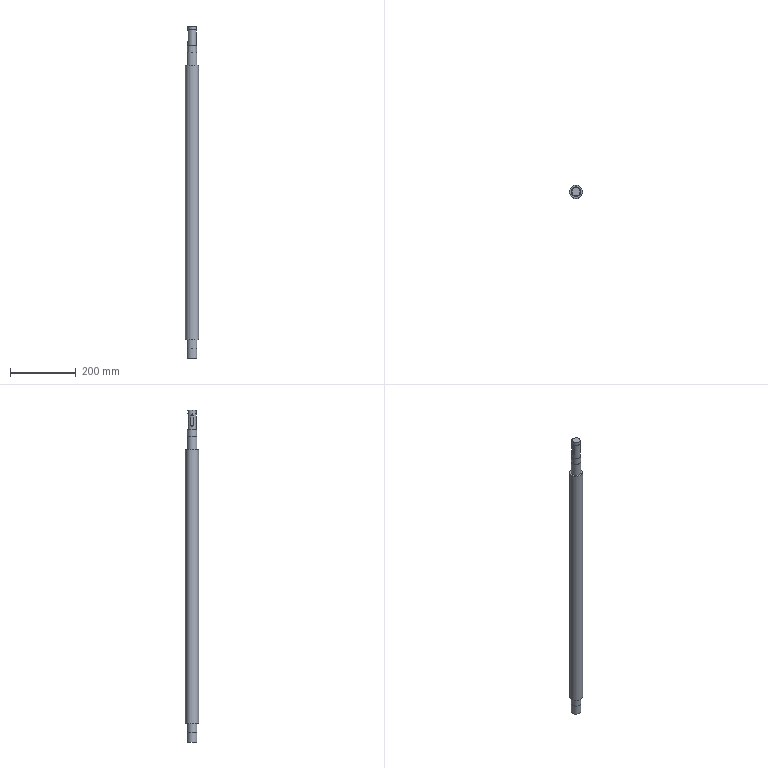Part | NX | features EXTRUDE 8, DATUM_CSYS 5, SKETCH 4, EXTRACT_DATUM_AXIS 2, CPROJ 1, DATUM_PLANE 1, EXTRACT_DATUM_PLANE 1, LINKED_POINT 1 | 3 solids | 24 faces | volume 1157120 mm3 | plane 14 | cylinder 10 | commonest cylinder face diameters 30 x3 8 x2 25 x2 23.2 x1 28 x1 40 x1
STEP:
#1=CARTESIAN_POINT('',(20.,0.,-405.));
#2=VERTEX_POINT('',#1);
#3=CARTESIAN_POINT('',(0.,0.,-405.));
#4=DIRECTION('',(0.,0.,1.));
#5=DIRECTION('',(1.,0.,0.));
#6=AXIS2_PLACEMENT_3D('',#3,#4,#5);
#7=CIRCLE('',#6,20.);
#8=EDGE_CURVE('',#2,#2,#7,.T.);
#9=ORIENTED_EDGE('',*,*,#8,.T.);
#10=EDGE_LOOP('',(#9));
#11=FACE_BOUND('',#10,.T.);
#12=CARTESIAN_POINT('',(20.,0.,430.));
#13=VERTEX_POINT('',#12);
#14=CARTESIAN_POINT('',(0.,0.,430.));
#15=DIRECTION('',(0.,0.,1.));
#16=DIRECTION('',(1.,0.,0.));
#17=AXIS2_PLACEMENT_3D('',#14,#15,#16);
#18=CIRCLE('',#17,20.);
#19=EDGE_CURVE('',#13,#13,#18,.T.);
#20=ORIENTED_EDGE('',*,*,#19,.F.);
#21=EDGE_LOOP('',(#20));
#22=FACE_BOUND('',#21,.T.);
#23=CARTESIAN_POINT('',(0.,0.,430.));
#24=DIRECTION('',(0.,0.,-1.));
#25=DIRECTION('',(-1.,0.,0.));
#26=AXIS2_PLACEMENT_3D('',#23,#24,#25);
#27=CYLINDRICAL_SURFACE('',#26,20.);
#28=ADVANCED_FACE('',(#11,#22),#27,.T.);
#29=ORIENTED_EDGE('',*,*,#19,.T.);
#30=EDGE_LOOP('',(#29));
#31=FACE_BOUND('',#30,.T.);
#32=CARTESIAN_POINT('',(0.,0.,430.));
#33=DIRECTION('',(0.,0.,1.));
#34=DIRECTION('',(1.,0.,0.));
#35=AXIS2_PLACEMENT_3D('',#32,#33,#34);
#36=PLANE('',#35);
#37=ADVANCED_FACE('',(#31),#36,.T.);
#38=CARTESIAN_POINT('',(-15.,0.,-405.));
#39=VERTEX_POINT('',#38);
#40=CARTESIAN_POINT('',(0.,0.,-405.));
#41=DIRECTION('',(0.,0.,-1.));
#42=DIRECTION('',(-1.,0.,0.));
#43=AXIS2_PLACEMENT_3D('',#40,#41,#42);
#44=CIRCLE('',#43,15.);
#45=EDGE_CURVE('',#39,#39,#44,.F.);
#46=ORIENTED_EDGE('',*,*,#45,.F.);
#47=EDGE_LOOP('',(#46));
#48=FACE_BOUND('',#47,.T.);
#49=CARTESIAN_POINT('',(-15.,0.,-430.));
#50=VERTEX_POINT('',#49);
#51=CARTESIAN_POINT('',(0.,0.,-430.));
#52=DIRECTION('',(0.,0.,-1.));
#53=DIRECTION('',(-1.,0.,0.));
#54=AXIS2_PLACEMENT_3D('',#51,#52,#53);
#55=CIRCLE('',#54,15.);
#56=EDGE_CURVE('',#50,#50,#55,.T.);
#57=ORIENTED_EDGE('',*,*,#56,.F.);
#58=EDGE_LOOP('',(#57));
#59=FACE_BOUND('',#58,.T.);
#60=CARTESIAN_POINT('',(0.,0.,-405.));
#61=DIRECTION('',(0.,0.,-1.));
#62=DIRECTION('',(-1.,0.,0.));
#63=AXIS2_PLACEMENT_3D('',#60,#61,#62);
#64=CYLINDRICAL_SURFACE('',#63,15.);
#65=ADVANCED_FACE('',(#48,#59),#64,.T.);
#66=ORIENTED_EDGE('',*,*,#8,.F.);
#67=EDGE_LOOP('',(#66));
#68=FACE_BOUND('',#67,.T.);
#69=ORIENTED_EDGE('',*,*,#45,.T.);
#70=EDGE_LOOP('',(#69));
#71=FACE_BOUND('',#70,.T.);
#72=CARTESIAN_POINT('',(0.,0.,-405.));
#73=DIRECTION('',(0.,0.,1.));
#74=DIRECTION('',(1.,0.,0.));
#75=AXIS2_PLACEMENT_3D('',#72,#73,#74);
#76=PLANE('',#75);
#77=ADVANCED_FACE('',(#68,#71),#76,.F.);
#78=ORIENTED_EDGE('',*,*,#56,.T.);
#79=EDGE_LOOP('',(#78));
#80=FACE_BOUND('',#79,.T.);
#81=CARTESIAN_POINT('',(0.,0.,-430.));
#82=DIRECTION('',(0.,0.,1.));
#83=DIRECTION('',(1.,0.,0.));
#84=AXIS2_PLACEMENT_3D('',#81,#82,#83);
#85=PLANE('',#84);
#86=ADVANCED_FACE('',(#80),#85,.F.);
#87=CLOSED_SHELL('',(#28,#37,#65,#77,#86));
#88=MANIFOLD_SOLID_BREP('',#87);
#89=CARTESIAN_POINT('',(-11.843,4.,505.));
#90=VERTEX_POINT('',#89);
#91=CARTESIAN_POINT('',(-11.843,-4.,505.));
#92=VERTEX_POINT('',#91);
#93=CARTESIAN_POINT('',(-11.843,4.,505.));
#94=CARTESIAN_POINT('',(-11.843,4.,503.936));
#95=CARTESIAN_POINT('',(-12.18,3.133,501.876));
#96=CARTESIAN_POINT('',(-12.66,0.006695,500.563));
#97=CARTESIAN_POINT('',(-12.181,-3.135,501.874));
#98=CARTESIAN_POINT('',(-11.843,-4.,503.936));
#99=CARTESIAN_POINT('',(-11.843,-4.,505.));
#100=B_SPLINE_CURVE_WITH_KNOTS('',3,(#93,#94,#95,#96,#97,#98,#99),.UNSPECIFIED.,.F.,.F.,(4,1,1,1,4),(0.,0.003146,0.006292,0.009438,0.01258),.UNSPECIFIED.);
#101=EDGE_CURVE('',#90,#92,#100,.T.);
#102=ORIENTED_EDGE('',*,*,#101,.F.);
#103=CARTESIAN_POINT('',(-11.843,4.,532.));
#104=VERTEX_POINT('',#103);
#105=CARTESIAN_POINT('',(-11.843,4.,550.));
#106=DIRECTION('',(0.,0.,-1.));
#107=VECTOR('',#106,1000.);
#108=LINE('',#105,#107);
#109=EDGE_CURVE('',#104,#90,#108,.T.);
#110=ORIENTED_EDGE('',*,*,#109,.F.);
#111=CARTESIAN_POINT('',(-11.843,-4.,532.));
#112=VERTEX_POINT('',#111);
#113=CARTESIAN_POINT('',(-11.843,-4.,532.));
#114=CARTESIAN_POINT('',(-11.843,-4.,533.064));
#115=CARTESIAN_POINT('',(-12.18,-3.133,535.124));
#116=CARTESIAN_POINT('',(-12.66,-0.006695,536.437));
#117=CARTESIAN_POINT('',(-12.181,3.135,535.126));
#118=CARTESIAN_POINT('',(-11.843,4.,533.064));
#119=CARTESIAN_POINT('',(-11.843,4.,532.));
#120=B_SPLINE_CURVE_WITH_KNOTS('',3,(#113,#114,#115,#116,#117,#118,#119),.UNSPECIFIED.,.F.,.F.,(4,1,1,1,4),(0.,0.003146,0.006292,0.009438,0.01258),.UNSPECIFIED.);
#121=EDGE_CURVE('',#112,#104,#120,.T.);
#122=ORIENTED_EDGE('',*,*,#121,.F.);
#123=CARTESIAN_POINT('',(-11.843,-4.,550.));
#124=DIRECTION('',(0.,0.,-1.));
#125=VECTOR('',#124,1000.);
#126=LINE('',#123,#125);
#127=EDGE_CURVE('',#92,#112,#126,.F.);
#128=ORIENTED_EDGE('',*,*,#127,.F.);
#129=EDGE_LOOP('',(#102,#110,#122,#128));
#130=FACE_BOUND('',#129,.T.);
#131=CARTESIAN_POINT('',(12.5,0.,490.));
#132=VERTEX_POINT('',#131);
#133=CARTESIAN_POINT('',(0.,0.,490.));
#134=DIRECTION('',(0.,0.,1.));
#135=DIRECTION('',(1.,0.,0.));
#136=AXIS2_PLACEMENT_3D('',#133,#134,#135);
#137=CIRCLE('',#136,12.5);
#138=EDGE_CURVE('',#132,#132,#137,.T.);
#139=ORIENTED_EDGE('',*,*,#138,.T.);
#140=EDGE_LOOP('',(#139));
#141=FACE_BOUND('',#140,.T.);
#142=CARTESIAN_POINT('',(12.5,0.,538.));
#143=VERTEX_POINT('',#142);
#144=CARTESIAN_POINT('',(0.,0.,538.));
#145=DIRECTION('',(0.,0.,1.));
#146=DIRECTION('',(1.,0.,0.));
#147=AXIS2_PLACEMENT_3D('',#144,#145,#146);
#148=CIRCLE('',#147,12.5);
#149=EDGE_CURVE('',#143,#143,#148,.T.);
#150=ORIENTED_EDGE('',*,*,#149,.F.);
#151=EDGE_LOOP('',(#150));
#152=FACE_BOUND('',#151,.T.);
#153=CARTESIAN_POINT('',(0.,0.,550.));
#154=DIRECTION('',(0.,0.,-1.));
#155=DIRECTION('',(-1.,0.,0.));
#156=AXIS2_PLACEMENT_3D('',#153,#154,#155);
#157=CYLINDRICAL_SURFACE('',#156,12.5);
#158=ADVANCED_FACE('',(#130,#141,#152),#157,.T.);
#159=CARTESIAN_POINT('',(14.,0.,490.));
#160=VERTEX_POINT('',#159);
#161=CARTESIAN_POINT('',(0.,0.,490.));
#162=DIRECTION('',(0.,0.,1.));
#163=DIRECTION('',(1.,0.,0.));
#164=AXIS2_PLACEMENT_3D('',#161,#162,#163);
#165=CIRCLE('',#164,14.);
#166=EDGE_CURVE('',#160,#160,#165,.T.);
#167=ORIENTED_EDGE('',*,*,#166,.F.);
#168=EDGE_LOOP('',(#167));
#169=FACE_BOUND('',#168,.T.);
#170=CARTESIAN_POINT('',(14.,0.,470.));
#171=VERTEX_POINT('',#170);
#172=CARTESIAN_POINT('',(0.,0.,470.));
#173=DIRECTION('',(0.,0.,1.));
#174=DIRECTION('',(1.,0.,0.));
#175=AXIS2_PLACEMENT_3D('',#172,#173,#174);
#176=CIRCLE('',#175,14.);
#177=EDGE_CURVE('',#171,#171,#176,.T.);
#178=ORIENTED_EDGE('',*,*,#177,.T.);
#179=EDGE_LOOP('',(#178));
#180=FACE_BOUND('',#179,.T.);
#181=CARTESIAN_POINT('',(0.,0.,490.));
#182=DIRECTION('',(0.,0.,-1.));
#183=DIRECTION('',(-1.,0.,0.));
#184=AXIS2_PLACEMENT_3D('',#181,#182,#183);
#185=CYLINDRICAL_SURFACE('',#184,14.);
#186=ADVANCED_FACE('',(#169,#180),#185,.T.);
#187=ORIENTED_EDGE('',*,*,#138,.F.);
#188=EDGE_LOOP('',(#187));
#189=FACE_BOUND('',#188,.T.);
#190=ORIENTED_EDGE('',*,*,#166,.T.);
#191=EDGE_LOOP('',(#190));
#192=FACE_BOUND('',#191,.T.);
#193=CARTESIAN_POINT('',(0.,0.,490.));
#194=DIRECTION('',(0.,0.,1.));
#195=DIRECTION('',(1.,0.,0.));
#196=AXIS2_PLACEMENT_3D('',#193,#194,#195);
#197=PLANE('',#196);
#198=ADVANCED_FACE('',(#189,#192),#197,.T.);
#199=CARTESIAN_POINT('',(15.,0.,470.));
#200=VERTEX_POINT('',#199);
#201=CARTESIAN_POINT('',(0.,0.,470.));
#202=DIRECTION('',(0.,0.,1.));
#203=DIRECTION('',(1.,0.,0.));
#204=AXIS2_PLACEMENT_3D('',#201,#202,#203);
#205=CIRCLE('',#204,15.);
#206=EDGE_CURVE('',#200,#200,#205,.T.);
#207=ORIENTED_EDGE('',*,*,#206,.F.);
#208=EDGE_LOOP('',(#207));
#209=FACE_BOUND('',#208,.T.);
#210=CARTESIAN_POINT('',(15.,0.,430.));
#211=VERTEX_POINT('',#210);
#212=CARTESIAN_POINT('',(0.,0.,430.));
#213=DIRECTION('',(0.,0.,1.));
#214=DIRECTION('',(1.,0.,0.));
#215=AXIS2_PLACEMENT_3D('',#212,#213,#214);
#216=CIRCLE('',#215,15.);
#217=EDGE_CURVE('',#211,#211,#216,.T.);
#218=ORIENTED_EDGE('',*,*,#217,.T.);
#219=EDGE_LOOP('',(#218));
#220=FACE_BOUND('',#219,.T.);
#221=CARTESIAN_POINT('',(0.,0.,470.));
#222=DIRECTION('',(0.,0.,-1.));
#223=DIRECTION('',(-1.,0.,0.));
#224=AXIS2_PLACEMENT_3D('',#221,#222,#223);
#225=CYLINDRICAL_SURFACE('',#224,15.);
#226=ADVANCED_FACE('',(#209,#220),#225,.T.);
#227=ORIENTED_EDGE('',*,*,#177,.F.);
#228=EDGE_LOOP('',(#227));
#229=FACE_BOUND('',#228,.T.);
#230=ORIENTED_EDGE('',*,*,#206,.T.);
#231=EDGE_LOOP('',(#230));
#232=FACE_BOUND('',#231,.T.);
#233=CARTESIAN_POINT('',(0.,0.,470.));
#234=DIRECTION('',(0.,0.,1.));
#235=DIRECTION('',(1.,0.,0.));
#236=AXIS2_PLACEMENT_3D('',#233,#234,#235);
#237=PLANE('',#236);
#238=ADVANCED_FACE('',(#229,#232),#237,.T.);
#239=ORIENTED_EDGE('',*,*,#217,.F.);
#240=EDGE_LOOP('',(#239));
#241=FACE_BOUND('',#240,.T.);
#242=CARTESIAN_POINT('',(0.,0.,430.));
#243=DIRECTION('',(0.,0.,1.));
#244=DIRECTION('',(1.,0.,0.));
#245=AXIS2_PLACEMENT_3D('',#242,#243,#244);
#246=PLANE('',#245);
#247=ADVANCED_FACE('',(#241),#246,.F.);
#248=CARTESIAN_POINT('',(-8.5,-4.,532.));
#249=VERTEX_POINT('',#248);
#250=CARTESIAN_POINT('',(-8.5,-4.,532.));
#251=DIRECTION('',(-1.,0.,0.));
#252=VECTOR('',#251,1000.);
#253=LINE('',#250,#252);
#254=EDGE_CURVE('',#112,#249,#253,.F.);
#255=ORIENTED_EDGE('',*,*,#254,.F.);
#256=ORIENTED_EDGE('',*,*,#121,.T.);
#257=CARTESIAN_POINT('',(-8.5,4.,532.));
#258=VERTEX_POINT('',#257);
#259=CARTESIAN_POINT('',(-8.5,4.,532.));
#260=DIRECTION('',(-1.,0.,0.));
#261=VECTOR('',#260,1000.);
#262=LINE('',#259,#261);
#263=EDGE_CURVE('',#104,#258,#262,.F.);
#264=ORIENTED_EDGE('',*,*,#263,.T.);
#265=CARTESIAN_POINT('',(-8.5,0.,532.));
#266=DIRECTION('',(1.,0.,0.));
#267=DIRECTION('',(0.,1.,0.));
#268=AXIS2_PLACEMENT_3D('',#265,#266,#267);
#269=CIRCLE('',#268,4.);
#270=EDGE_CURVE('',#249,#258,#269,.F.);
#271=ORIENTED_EDGE('',*,*,#270,.F.);
#272=EDGE_LOOP('',(#255,#256,#264,#271));
#273=FACE_BOUND('',#272,.T.);
#274=CARTESIAN_POINT('',(-8.5,0.,532.));
#275=DIRECTION('',(-1.,0.,0.));
#276=DIRECTION('',(0.,0.,1.));
#277=AXIS2_PLACEMENT_3D('',#274,#275,#276);
#278=CYLINDRICAL_SURFACE('',#277,4.);
#279=ADVANCED_FACE('',(#273),#278,.F.);
#280=ORIENTED_EDGE('',*,*,#127,.T.);
#281=ORIENTED_EDGE('',*,*,#254,.T.);
#282=CARTESIAN_POINT('',(-8.5,-4.,505.));
#283=VERTEX_POINT('',#282);
#284=CARTESIAN_POINT('',(-8.5,-4.,532.));
#285=DIRECTION('',(0.,0.,-1.));
#286=VECTOR('',#285,1000.);
#287=LINE('',#284,#286);
#288=EDGE_CURVE('',#283,#249,#287,.F.);
#289=ORIENTED_EDGE('',*,*,#288,.F.);
#290=CARTESIAN_POINT('',(-8.5,-4.,505.));
#291=DIRECTION('',(-1.,0.,0.));
#292=VECTOR('',#291,1000.);
#293=LINE('',#290,#292);
#294=EDGE_CURVE('',#92,#283,#293,.F.);
#295=ORIENTED_EDGE('',*,*,#294,.F.);
#296=EDGE_LOOP('',(#280,#281,#289,#295));
#297=FACE_BOUND('',#296,.T.);
#298=CARTESIAN_POINT('',(-8.5,-4.,532.));
#299=DIRECTION('',(0.,1.,0.));
#300=DIRECTION('',(0.,0.,1.));
#301=AXIS2_PLACEMENT_3D('',#298,#299,#300);
#302=PLANE('',#301);
#303=ADVANCED_FACE('',(#297),#302,.T.);
#304=CARTESIAN_POINT('',(-8.5,4.,505.));
#305=VERTEX_POINT('',#304);
#306=CARTESIAN_POINT('',(-8.5,4.,505.));
#307=DIRECTION('',(-1.,0.,0.));
#308=VECTOR('',#307,1000.);
#309=LINE('',#306,#308);
#310=EDGE_CURVE('',#90,#305,#309,.F.);
#311=ORIENTED_EDGE('',*,*,#310,.F.);
#312=ORIENTED_EDGE('',*,*,#101,.T.);
#313=ORIENTED_EDGE('',*,*,#294,.T.);
#314=CARTESIAN_POINT('',(-8.5,0.,505.));
#315=DIRECTION('',(1.,0.,0.));
#316=DIRECTION('',(0.,1.,0.));
#317=AXIS2_PLACEMENT_3D('',#314,#315,#316);
#318=CIRCLE('',#317,4.);
#319=EDGE_CURVE('',#305,#283,#318,.F.);
#320=ORIENTED_EDGE('',*,*,#319,.F.);
#321=EDGE_LOOP('',(#311,#312,#313,#320));
#322=FACE_BOUND('',#321,.T.);
#323=CARTESIAN_POINT('',(-8.5,0.,505.));
#324=DIRECTION('',(-1.,0.,0.));
#325=DIRECTION('',(0.,0.,1.));
#326=AXIS2_PLACEMENT_3D('',#323,#324,#325);
#327=CYLINDRICAL_SURFACE('',#326,4.);
#328=ADVANCED_FACE('',(#322),#327,.F.);
#329=ORIENTED_EDGE('',*,*,#109,.T.);
#330=ORIENTED_EDGE('',*,*,#310,.T.);
#331=CARTESIAN_POINT('',(-8.5,4.,505.));
#332=DIRECTION('',(0.,0.,1.));
#333=VECTOR('',#332,1000.);
#334=LINE('',#331,#333);
#335=EDGE_CURVE('',#258,#305,#334,.F.);
#336=ORIENTED_EDGE('',*,*,#335,.F.);
#337=ORIENTED_EDGE('',*,*,#263,.F.);
#338=EDGE_LOOP('',(#329,#330,#336,#337));
#339=FACE_BOUND('',#338,.T.);
#340=CARTESIAN_POINT('',(-8.5,4.,505.));
#341=DIRECTION('',(0.,-1.,0.));
#342=DIRECTION('',(0.,0.,-1.));
#343=AXIS2_PLACEMENT_3D('',#340,#341,#342);
#344=PLANE('',#343);
#345=ADVANCED_FACE('',(#339),#344,.T.);
#346=ORIENTED_EDGE('',*,*,#270,.T.);
#347=ORIENTED_EDGE('',*,*,#335,.T.);
#348=ORIENTED_EDGE('',*,*,#319,.T.);
#349=ORIENTED_EDGE('',*,*,#288,.T.);
#350=EDGE_LOOP('',(#346,#347,#348,#349));
#351=FACE_BOUND('',#350,.T.);
#352=CARTESIAN_POINT('',(-8.5,0.,532.));
#353=DIRECTION('',(1.,0.,0.));
#354=DIRECTION('',(0.,0.,-1.));
#355=AXIS2_PLACEMENT_3D('',#352,#353,#354);
#356=PLANE('',#355);
#357=ADVANCED_FACE('',(#351),#356,.F.);
#358=CARTESIAN_POINT('',(11.6,0.,539.2));
#359=VERTEX_POINT('',#358);
#360=CARTESIAN_POINT('',(0.,0.,539.2));
#361=DIRECTION('',(0.,0.,1.));
#362=DIRECTION('',(1.,0.,0.));
#363=AXIS2_PLACEMENT_3D('',#360,#361,#362);
#364=CIRCLE('',#363,11.6);
#365=EDGE_CURVE('',#359,#359,#364,.F.);
#366=ORIENTED_EDGE('',*,*,#365,.F.);
#367=EDGE_LOOP('',(#366));
#368=FACE_BOUND('',#367,.T.);
#369=CARTESIAN_POINT('',(12.5,0.,539.2));
#370=VERTEX_POINT('',#369);
#371=CARTESIAN_POINT('',(0.,0.,539.2));
#372=DIRECTION('',(0.,0.,1.));
#373=DIRECTION('',(1.,0.,0.));
#374=AXIS2_PLACEMENT_3D('',#371,#372,#373);
#375=CIRCLE('',#374,12.5);
#376=EDGE_CURVE('',#370,#370,#375,.T.);
#377=ORIENTED_EDGE('',*,*,#376,.F.);
#378=EDGE_LOOP('',(#377));
#379=FACE_BOUND('',#378,.T.);
#380=CARTESIAN_POINT('',(0.,0.,539.2));
#381=DIRECTION('',(0.,0.,1.));
#382=DIRECTION('',(1.,0.,0.));
#383=AXIS2_PLACEMENT_3D('',#380,#381,#382);
#384=PLANE('',#383);
#385=ADVANCED_FACE('',(#368,#379),#384,.F.);
#386=CARTESIAN_POINT('',(11.6,0.,538.));
#387=VERTEX_POINT('',#386);
#388=CARTESIAN_POINT('',(0.,0.,538.));
#389=DIRECTION('',(0.,0.,1.));
#390=DIRECTION('',(1.,0.,0.));
#391=AXIS2_PLACEMENT_3D('',#388,#389,#390);
#392=CIRCLE('',#391,11.6);
#393=EDGE_CURVE('',#387,#387,#392,.F.);
#394=ORIENTED_EDGE('',*,*,#393,.T.);
#395=EDGE_LOOP('',(#394));
#396=FACE_BOUND('',#395,.T.);
#397=ORIENTED_EDGE('',*,*,#149,.T.);
#398=EDGE_LOOP('',(#397));
#399=FACE_BOUND('',#398,.T.);
#400=CARTESIAN_POINT('',(0.,0.,538.));
#401=DIRECTION('',(0.,0.,1.));
#402=DIRECTION('',(1.,0.,0.));
#403=AXIS2_PLACEMENT_3D('',#400,#401,#402);
#404=PLANE('',#403);
#405=ADVANCED_FACE('',(#396,#399),#404,.T.);
#406=ORIENTED_EDGE('',*,*,#365,.T.);
#407=EDGE_LOOP('',(#406));
#408=FACE_BOUND('',#407,.T.);
#409=ORIENTED_EDGE('',*,*,#393,.F.);
#410=EDGE_LOOP('',(#409));
#411=FACE_BOUND('',#410,.T.);
#412=CARTESIAN_POINT('',(0.,0.,539.2));
#413=DIRECTION('',(0.,0.,-1.));
#414=DIRECTION('',(-1.,0.,0.));
#415=AXIS2_PLACEMENT_3D('',#412,#413,#414);
#416=CYLINDRICAL_SURFACE('',#415,11.6);
#417=ADVANCED_FACE('',(#408,#411),#416,.T.);
#418=CARTESIAN_POINT('',(12.5,0.,550.));
#419=VERTEX_POINT('',#418);
#420=CARTESIAN_POINT('',(0.,0.,550.));
#421=DIRECTION('',(0.,0.,1.));
#422=DIRECTION('',(1.,0.,0.));
#423=AXIS2_PLACEMENT_3D('',#420,#421,#422);
#424=CIRCLE('',#423,12.5);
#425=EDGE_CURVE('',#419,#419,#424,.T.);
#426=ORIENTED_EDGE('',*,*,#425,.T.);
#427=EDGE_LOOP('',(#426));
#428=FACE_BOUND('',#427,.T.);
#429=CARTESIAN_POINT('',(0.,0.,550.));
#430=DIRECTION('',(0.,0.,1.));
#431=DIRECTION('',(1.,0.,0.));
#432=AXIS2_PLACEMENT_3D('',#429,#430,#431);
#433=PLANE('',#432);
#434=ADVANCED_FACE('',(#428),#433,.T.);
#435=ORIENTED_EDGE('',*,*,#376,.T.);
#436=EDGE_LOOP('',(#435));
#437=FACE_BOUND('',#436,.T.);
#438=ORIENTED_EDGE('',*,*,#425,.F.);
#439=EDGE_LOOP('',(#438));
#440=FACE_BOUND('',#439,.T.);
#441=CARTESIAN_POINT('',(0.,0.,550.));
#442=DIRECTION('',(0.,0.,-1.));
#443=DIRECTION('',(-1.,0.,0.));
#444=AXIS2_PLACEMENT_3D('',#441,#442,#443);
#445=CYLINDRICAL_SURFACE('',#444,12.5);
#446=ADVANCED_FACE('',(#437,#440),#445,.T.);
#447=CLOSED_SHELL('',(#158,#186,#198,#226,#238,#247,#279,#303,#328,#345,#357,#385,#405,#417,#434,#446));
#448=MANIFOLD_SOLID_BREP('',#447);
#449=CARTESIAN_POINT('',(15.,0.,-460.));
#450=VERTEX_POINT('',#449);
#451=CARTESIAN_POINT('',(0.,0.,-460.));
#452=DIRECTION('',(0.,0.,1.));
#453=DIRECTION('',(1.,0.,0.));
#454=AXIS2_PLACEMENT_3D('',#451,#452,#453);
#455=CIRCLE('',#454,15.);
#456=EDGE_CURVE('',#450,#450,#455,.T.);
#457=ORIENTED_EDGE('',*,*,#456,.T.);
#458=EDGE_LOOP('',(#457));
#459=FACE_BOUND('',#458,.T.);
#460=CARTESIAN_POINT('',(15.,0.,-430.));
#461=VERTEX_POINT('',#460);
#462=CARTESIAN_POINT('',(0.,0.,-430.));
#463=DIRECTION('',(0.,0.,1.));
#464=DIRECTION('',(1.,0.,0.));
#465=AXIS2_PLACEMENT_3D('',#462,#463,#464);
#466=CIRCLE('',#465,15.);
#467=EDGE_CURVE('',#461,#461,#466,.T.);
#468=ORIENTED_EDGE('',*,*,#467,.F.);
#469=EDGE_LOOP('',(#468));
#470=FACE_BOUND('',#469,.T.);
#471=CARTESIAN_POINT('',(0.,0.,-460.));
#472=DIRECTION('',(0.,0.,1.));
#473=DIRECTION('',(1.,0.,0.));
#474=AXIS2_PLACEMENT_3D('',#471,#472,#473);
#475=CYLINDRICAL_SURFACE('',#474,15.);
#476=ADVANCED_FACE('',(#459,#470),#475,.T.);
#477=ORIENTED_EDGE('',*,*,#456,.F.);
#478=EDGE_LOOP('',(#477));
#479=FACE_BOUND('',#478,.T.);
#480=CARTESIAN_POINT('',(0.,0.,-460.));
#481=DIRECTION('',(0.,0.,1.));
#482=DIRECTION('',(1.,0.,0.));
#483=AXIS2_PLACEMENT_3D('',#480,#481,#482);
#484=PLANE('',#483);
#485=ADVANCED_FACE('',(#479),#484,.F.);
#486=ORIENTED_EDGE('',*,*,#467,.T.);
#487=EDGE_LOOP('',(#486));
#488=FACE_BOUND('',#487,.T.);
#489=CARTESIAN_POINT('',(0.,0.,-430.));
#490=DIRECTION('',(0.,0.,1.));
#491=DIRECTION('',(1.,0.,0.));
#492=AXIS2_PLACEMENT_3D('',#489,#490,#491);
#493=PLANE('',#492);
#494=ADVANCED_FACE('',(#488),#493,.T.);
#495=CLOSED_SHELL('',(#476,#485,#494));
#496=MANIFOLD_SOLID_BREP('',#495);
#497=(LENGTH_UNIT()NAMED_UNIT(*)SI_UNIT(.MILLI.,.METRE.));
#498=UNCERTAINTY_MEASURE_WITH_UNIT(LENGTH_MEASURE(0.0508),#497,'','');
#499=(NAMED_UNIT(*)PLANE_ANGLE_UNIT()SI_UNIT($,.RADIAN.));
#500=(NAMED_UNIT(*)SI_UNIT($,.STERADIAN.)SOLID_ANGLE_UNIT());
#501=(GEOMETRIC_REPRESENTATION_CONTEXT(3)GLOBAL_UNCERTAINTY_ASSIGNED_CONTEXT((#498))GLOBAL_UNIT_ASSIGNED_CONTEXT((#497,#499,#500))REPRESENTATION_CONTEXT('',''));
#502=ADVANCED_BREP_SHAPE_REPRESENTATION('',(#88,#448,#496),#501);